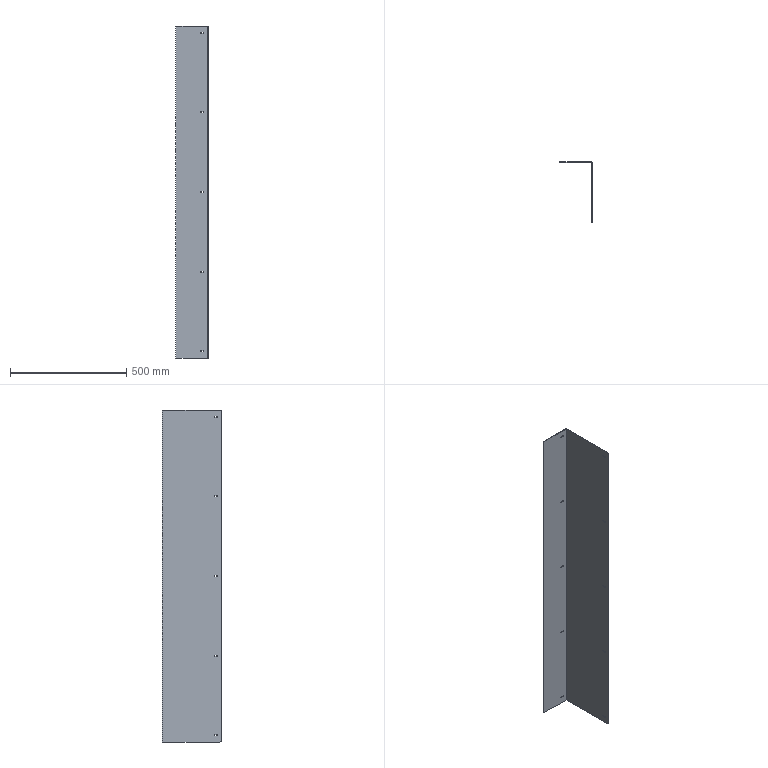Part | SolidWorks | features BaseBody 1 | 1 solid | 52 faces | box 138.931 x 257 x 1427 mm | volume 1121398 mm3 | plane 28 | cylinder 24 | commonest cylinder face diameters 4.3 x10 5.3 x10 20 x2 0.4 x1 4.4 x1